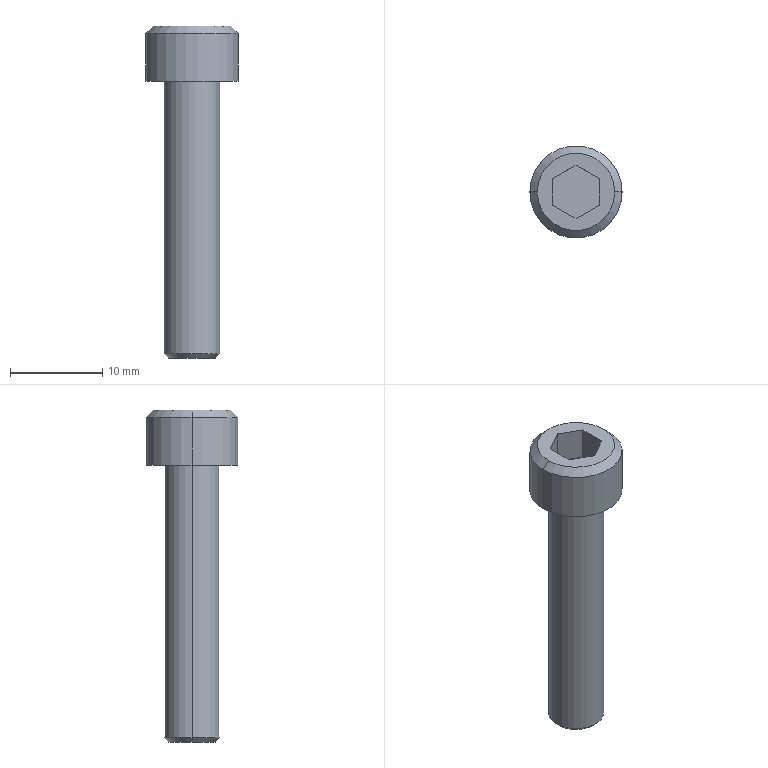Part | Creo | 1 solid | 18 faces | box 10 x 10 x 36 mm | volume 1230 mm3 | plane 10 | cylinder 4 | cone 4 | commonest cylinder face diameters 6 x2 10 x2
STEP:
#1=CARTESIAN_POINT('',(116.735,-194.,47.5));
#2=VERTEX_POINT('',#1);
#3=CARTESIAN_POINT('',(106.735,-194.,47.5));
#4=VERTEX_POINT('',#3);
#5=CARTESIAN_POINT('',(111.735,-194.,47.5));
#6=DIRECTION('',(0.,0.,-1.));
#7=DIRECTION('',(1.,0.,0.));
#8=AXIS2_PLACEMENT_3D('',#5,#6,#7);
#9=CIRCLE('',#8,5.);
#10=EDGE_CURVE('',#2,#4,#9,.T.);
#11=ORIENTED_EDGE('',*,*,#10,.F.);
#12=CARTESIAN_POINT('',(111.735,-194.,47.5));
#13=DIRECTION('',(0.,0.,-1.));
#14=DIRECTION('',(-1.,0.,0.));
#15=AXIS2_PLACEMENT_3D('',#12,#13,#14);
#16=CIRCLE('',#15,5.);
#17=EDGE_CURVE('',#4,#2,#16,.T.);
#18=ORIENTED_EDGE('',*,*,#17,.F.);
#19=EDGE_LOOP('',(#11,#18));
#20=FACE_OUTER_BOUND('',#19,.F.);
#21=CARTESIAN_POINT('',(108.735,-194.,47.5));
#22=VERTEX_POINT('',#21);
#23=CARTESIAN_POINT('',(114.735,-194.,47.5));
#24=VERTEX_POINT('',#23);
#25=CARTESIAN_POINT('',(111.735,-194.,47.5));
#26=DIRECTION('',(0.,0.,1.));
#27=DIRECTION('',(-1.,0.,0.));
#28=AXIS2_PLACEMENT_3D('',#25,#26,#27);
#29=CIRCLE('',#28,3.);
#30=EDGE_CURVE('',#22,#24,#29,.T.);
#31=ORIENTED_EDGE('',*,*,#30,.F.);
#32=CARTESIAN_POINT('',(111.735,-194.,47.5));
#33=DIRECTION('',(0.,0.,1.));
#34=DIRECTION('',(1.,0.,0.));
#35=AXIS2_PLACEMENT_3D('',#32,#33,#34);
#36=CIRCLE('',#35,3.);
#37=EDGE_CURVE('',#24,#22,#36,.T.);
#38=ORIENTED_EDGE('',*,*,#37,.F.);
#39=EDGE_LOOP('',(#31,#38));
#40=FACE_BOUND('',#39,.F.);
#41=CARTESIAN_POINT('',(111.735,-194.,47.5));
#42=DIRECTION('',(0.,0.,-1.));
#43=DIRECTION('',(-1.,0.,0.));
#44=AXIS2_PLACEMENT_3D('',#41,#42,#43);
#45=PLANE('',#44);
#46=ADVANCED_FACE('',(#20,#40),#45,.T.);
#47=CARTESIAN_POINT('',(114.735,-194.,17.95));
#48=VERTEX_POINT('',#47);
#49=CARTESIAN_POINT('',(108.735,-194.,17.95));
#50=VERTEX_POINT('',#49);
#51=CARTESIAN_POINT('',(111.735,-194.,17.95));
#52=DIRECTION('',(0.,0.,-1.));
#53=DIRECTION('',(1.,0.,0.));
#54=AXIS2_PLACEMENT_3D('',#51,#52,#53);
#55=CIRCLE('',#54,3.);
#56=EDGE_CURVE('',#48,#50,#55,.T.);
#57=ORIENTED_EDGE('',*,*,#56,.T.);
#58=CARTESIAN_POINT('',(108.735,-194.,47.5));
#59=DIRECTION('',(0.,0.,-1.));
#60=VECTOR('',#59,29.55);
#61=LINE('',#58,#60);
#62=EDGE_CURVE('',#22,#50,#61,.T.);
#63=ORIENTED_EDGE('',*,*,#62,.F.);
#64=ORIENTED_EDGE('',*,*,#30,.T.);
#65=CARTESIAN_POINT('',(114.735,-194.,47.5));
#66=DIRECTION('',(0.,0.,-1.));
#67=VECTOR('',#66,29.55);
#68=LINE('',#65,#67);
#69=EDGE_CURVE('',#24,#48,#68,.T.);
#70=ORIENTED_EDGE('',*,*,#69,.T.);
#71=EDGE_LOOP('',(#57,#63,#64,#70));
#72=FACE_OUTER_BOUND('',#71,.F.);
#73=CARTESIAN_POINT('',(111.735,-194.,54.5));
#74=DIRECTION('',(0.,0.,-1.));
#75=DIRECTION('',(-1.,0.,0.));
#76=AXIS2_PLACEMENT_3D('',#73,#74,#75);
#77=CYLINDRICAL_SURFACE('',#76,3.);
#78=ADVANCED_FACE('',(#72),#77,.T.);
#79=CARTESIAN_POINT('',(114.285,-194.,17.5));
#80=VERTEX_POINT('',#79);
#81=CARTESIAN_POINT('',(109.185,-194.,17.5));
#82=VERTEX_POINT('',#81);
#83=CARTESIAN_POINT('',(111.735,-194.,17.5));
#84=DIRECTION('',(0.,0.,-1.));
#85=DIRECTION('',(1.,0.,0.));
#86=AXIS2_PLACEMENT_3D('',#83,#84,#85);
#87=CIRCLE('',#86,2.55);
#88=EDGE_CURVE('',#80,#82,#87,.T.);
#89=ORIENTED_EDGE('',*,*,#88,.T.);
#90=CARTESIAN_POINT('',(109.185,-194.,17.5));
#91=DIRECTION('',(-0.7071,0.,0.7071));
#92=VECTOR('',#91,0.6364);
#93=LINE('',#90,#92);
#94=EDGE_CURVE('',#82,#50,#93,.T.);
#95=ORIENTED_EDGE('',*,*,#94,.T.);
#96=ORIENTED_EDGE('',*,*,#56,.F.);
#97=CARTESIAN_POINT('',(114.285,-194.,17.5));
#98=DIRECTION('',(0.7071,0.,0.7071));
#99=VECTOR('',#98,0.6364);
#100=LINE('',#97,#99);
#101=EDGE_CURVE('',#80,#48,#100,.T.);
#102=ORIENTED_EDGE('',*,*,#101,.F.);
#103=EDGE_LOOP('',(#89,#95,#96,#102));
#104=FACE_OUTER_BOUND('',#103,.F.);
#105=CARTESIAN_POINT('',(111.735,-194.,17.725));
#106=DIRECTION('',(0.,0.,1.));
#107=DIRECTION('',(1.,0.,0.));
#108=AXIS2_PLACEMENT_3D('',#105,#106,#107);
#109=CONICAL_SURFACE('',#108,2.775,45.);
#110=ADVANCED_FACE('',(#104),#109,.T.);
#111=CARTESIAN_POINT('',(111.735,-194.,17.5));
#112=DIRECTION('',(0.,0.,-1.));
#113=DIRECTION('',(-1.,0.,0.));
#114=AXIS2_PLACEMENT_3D('',#111,#112,#113);
#115=CIRCLE('',#114,2.55);
#116=EDGE_CURVE('',#82,#80,#115,.T.);
#117=ORIENTED_EDGE('',*,*,#116,.F.);
#118=ORIENTED_EDGE('',*,*,#88,.F.);
#119=EDGE_LOOP('',(#117,#118));
#120=FACE_OUTER_BOUND('',#119,.F.);
#121=CARTESIAN_POINT('',(111.735,-194.,17.5));
#122=DIRECTION('',(0.,0.,-1.));
#123=DIRECTION('',(-1.,0.,0.));
#124=AXIS2_PLACEMENT_3D('',#121,#122,#123);
#125=PLANE('',#124);
#126=ADVANCED_FACE('',(#120),#125,.T.);
#127=ORIENTED_EDGE('',*,*,#116,.T.);
#128=ORIENTED_EDGE('',*,*,#101,.T.);
#129=CARTESIAN_POINT('',(111.735,-194.,17.95));
#130=DIRECTION('',(0.,0.,-1.));
#131=DIRECTION('',(-1.,0.,0.));
#132=AXIS2_PLACEMENT_3D('',#129,#130,#131);
#133=CIRCLE('',#132,3.);
#134=EDGE_CURVE('',#50,#48,#133,.T.);
#135=ORIENTED_EDGE('',*,*,#134,.F.);
#136=ORIENTED_EDGE('',*,*,#94,.F.);
#137=EDGE_LOOP('',(#127,#128,#135,#136));
#138=FACE_OUTER_BOUND('',#137,.F.);
#139=CARTESIAN_POINT('',(111.735,-194.,17.725));
#140=DIRECTION('',(0.,0.,1.));
#141=DIRECTION('',(1.,0.,0.));
#142=AXIS2_PLACEMENT_3D('',#139,#140,#141);
#143=CONICAL_SURFACE('',#142,2.775,45.);
#144=ADVANCED_FACE('',(#138),#143,.T.);
#145=ORIENTED_EDGE('',*,*,#134,.T.);
#146=ORIENTED_EDGE('',*,*,#69,.F.);
#147=ORIENTED_EDGE('',*,*,#37,.T.);
#148=ORIENTED_EDGE('',*,*,#62,.T.);
#149=EDGE_LOOP('',(#145,#146,#147,#148));
#150=FACE_OUTER_BOUND('',#149,.F.);
#151=CARTESIAN_POINT('',(111.735,-194.,54.5));
#152=DIRECTION('',(0.,0.,-1.));
#153=DIRECTION('',(-1.,0.,0.));
#154=AXIS2_PLACEMENT_3D('',#151,#152,#153);
#155=CYLINDRICAL_SURFACE('',#154,3.);
#156=ADVANCED_FACE('',(#150),#155,.T.);
#157=CARTESIAN_POINT('',(106.735,-194.,52.7));
#158=VERTEX_POINT('',#157);
#159=CARTESIAN_POINT('',(116.735,-194.,52.7));
#160=VERTEX_POINT('',#159);
#161=CARTESIAN_POINT('',(111.735,-194.,52.7));
#162=DIRECTION('',(0.,0.,1.));
#163=DIRECTION('',(-1.,0.,0.));
#164=AXIS2_PLACEMENT_3D('',#161,#162,#163);
#165=CIRCLE('',#164,5.);
#166=EDGE_CURVE('',#158,#160,#165,.T.);
#167=ORIENTED_EDGE('',*,*,#166,.T.);
#168=CARTESIAN_POINT('',(116.735,-194.,52.7));
#169=DIRECTION('',(0.,0.,-1.));
#170=VECTOR('',#169,5.2);
#171=LINE('',#168,#170);
#172=EDGE_CURVE('',#160,#2,#171,.T.);
#173=ORIENTED_EDGE('',*,*,#172,.T.);
#174=ORIENTED_EDGE('',*,*,#10,.T.);
#175=CARTESIAN_POINT('',(106.735,-194.,52.7));
#176=DIRECTION('',(0.,0.,-1.));
#177=VECTOR('',#176,5.2);
#178=LINE('',#175,#177);
#179=EDGE_CURVE('',#158,#4,#178,.T.);
#180=ORIENTED_EDGE('',*,*,#179,.F.);
#181=EDGE_LOOP('',(#167,#173,#174,#180));
#182=FACE_OUTER_BOUND('',#181,.F.);
#183=CARTESIAN_POINT('',(111.735,-194.,54.5));
#184=DIRECTION('',(0.,0.,-1.));
#185=DIRECTION('',(-1.,0.,0.));
#186=AXIS2_PLACEMENT_3D('',#183,#184,#185);
#187=CYLINDRICAL_SURFACE('',#186,5.);
#188=ADVANCED_FACE('',(#182),#187,.T.);
#189=CARTESIAN_POINT('',(107.535,-194.,53.5));
#190=VERTEX_POINT('',#189);
#191=CARTESIAN_POINT('',(115.935,-194.,53.5));
#192=VERTEX_POINT('',#191);
#193=CARTESIAN_POINT('',(111.735,-194.,53.5));
#194=DIRECTION('',(0.,0.,1.));
#195=DIRECTION('',(-1.,0.,0.));
#196=AXIS2_PLACEMENT_3D('',#193,#194,#195);
#197=CIRCLE('',#196,4.2);
#198=EDGE_CURVE('',#190,#192,#197,.T.);
#199=ORIENTED_EDGE('',*,*,#198,.T.);
#200=CARTESIAN_POINT('',(115.935,-194.,53.5));
#201=DIRECTION('',(0.7071,0.,-0.7071));
#202=VECTOR('',#201,1.131);
#203=LINE('',#200,#202);
#204=EDGE_CURVE('',#192,#160,#203,.T.);
#205=ORIENTED_EDGE('',*,*,#204,.T.);
#206=ORIENTED_EDGE('',*,*,#166,.F.);
#207=CARTESIAN_POINT('',(107.535,-194.,53.5));
#208=DIRECTION('',(-0.7071,0.,-0.7071));
#209=VECTOR('',#208,1.131);
#210=LINE('',#207,#209);
#211=EDGE_CURVE('',#190,#158,#210,.T.);
#212=ORIENTED_EDGE('',*,*,#211,.F.);
#213=EDGE_LOOP('',(#199,#205,#206,#212));
#214=FACE_OUTER_BOUND('',#213,.F.);
#215=CARTESIAN_POINT('',(111.735,-194.,53.1));
#216=DIRECTION('',(0.,0.,-1.));
#217=DIRECTION('',(-1.,0.,0.));
#218=AXIS2_PLACEMENT_3D('',#215,#216,#217);
#219=CONICAL_SURFACE('',#218,4.6,45.);
#220=ADVANCED_FACE('',(#214),#219,.T.);
#221=ORIENTED_EDGE('',*,*,#198,.F.);
#222=CARTESIAN_POINT('',(111.735,-194.,53.5));
#223=DIRECTION('',(0.,0.,1.));
#224=DIRECTION('',(1.,0.,0.));
#225=AXIS2_PLACEMENT_3D('',#222,#223,#224);
#226=CIRCLE('',#225,4.2);
#227=EDGE_CURVE('',#192,#190,#226,.T.);
#228=ORIENTED_EDGE('',*,*,#227,.F.);
#229=EDGE_LOOP('',(#221,#228));
#230=FACE_OUTER_BOUND('',#229,.F.);
#231=CARTESIAN_POINT('',(114.235,-195.443,53.5));
#232=VERTEX_POINT('',#231);
#233=CARTESIAN_POINT('',(111.735,-196.887,53.5));
#234=VERTEX_POINT('',#233);
#235=CARTESIAN_POINT('',(114.235,-195.443,53.5));
#236=DIRECTION('',(-0.866,-0.5,0.));
#237=VECTOR('',#236,2.887);
#238=LINE('',#235,#237);
#239=EDGE_CURVE('',#232,#234,#238,.T.);
#240=ORIENTED_EDGE('',*,*,#239,.F.);
#241=CARTESIAN_POINT('',(114.235,-192.557,53.5));
#242=VERTEX_POINT('',#241);
#243=CARTESIAN_POINT('',(114.235,-192.557,53.5));
#244=DIRECTION('',(0.,-1.,0.));
#245=VECTOR('',#244,2.887);
#246=LINE('',#243,#245);
#247=EDGE_CURVE('',#242,#232,#246,.T.);
#248=ORIENTED_EDGE('',*,*,#247,.F.);
#249=CARTESIAN_POINT('',(111.735,-191.113,53.5));
#250=VERTEX_POINT('',#249);
#251=CARTESIAN_POINT('',(111.735,-191.113,53.5));
#252=DIRECTION('',(0.866,-0.5,0.));
#253=VECTOR('',#252,2.887);
#254=LINE('',#251,#253);
#255=EDGE_CURVE('',#250,#242,#254,.T.);
#256=ORIENTED_EDGE('',*,*,#255,.F.);
#257=CARTESIAN_POINT('',(109.235,-192.557,53.5));
#258=VERTEX_POINT('',#257);
#259=CARTESIAN_POINT('',(109.235,-192.557,53.5));
#260=DIRECTION('',(0.866,0.5,0.));
#261=VECTOR('',#260,2.887);
#262=LINE('',#259,#261);
#263=EDGE_CURVE('',#258,#250,#262,.T.);
#264=ORIENTED_EDGE('',*,*,#263,.F.);
#265=CARTESIAN_POINT('',(109.235,-195.443,53.5));
#266=VERTEX_POINT('',#265);
#267=CARTESIAN_POINT('',(109.235,-195.443,53.5));
#268=DIRECTION('',(0.,1.,0.));
#269=VECTOR('',#268,2.887);
#270=LINE('',#267,#269);
#271=EDGE_CURVE('',#266,#258,#270,.T.);
#272=ORIENTED_EDGE('',*,*,#271,.F.);
#273=CARTESIAN_POINT('',(111.735,-196.887,53.5));
#274=DIRECTION('',(-0.866,0.5,0.));
#275=VECTOR('',#274,2.887);
#276=LINE('',#273,#275);
#277=EDGE_CURVE('',#234,#266,#276,.T.);
#278=ORIENTED_EDGE('',*,*,#277,.F.);
#279=EDGE_LOOP('',(#240,#248,#256,#264,#272,#278));
#280=FACE_BOUND('',#279,.F.);
#281=CARTESIAN_POINT('',(111.735,-194.,53.5));
#282=DIRECTION('',(0.,0.,-1.));
#283=DIRECTION('',(-1.,0.,0.));
#284=AXIS2_PLACEMENT_3D('',#281,#282,#283);
#285=PLANE('',#284);
#286=ADVANCED_FACE('',(#230,#280),#285,.F.);
#287=ORIENTED_EDGE('',*,*,#227,.T.);
#288=ORIENTED_EDGE('',*,*,#211,.T.);
#289=CARTESIAN_POINT('',(111.735,-194.,52.7));
#290=DIRECTION('',(0.,0.,1.));
#291=DIRECTION('',(1.,0.,0.));
#292=AXIS2_PLACEMENT_3D('',#289,#290,#291);
#293=CIRCLE('',#292,5.);
#294=EDGE_CURVE('',#160,#158,#293,.T.);
#295=ORIENTED_EDGE('',*,*,#294,.F.);
#296=ORIENTED_EDGE('',*,*,#204,.F.);
#297=EDGE_LOOP('',(#287,#288,#295,#296));
#298=FACE_OUTER_BOUND('',#297,.F.);
#299=CARTESIAN_POINT('',(111.735,-194.,53.1));
#300=DIRECTION('',(0.,0.,-1.));
#301=DIRECTION('',(-1.,0.,0.));
#302=AXIS2_PLACEMENT_3D('',#299,#300,#301);
#303=CONICAL_SURFACE('',#302,4.6,45.);
#304=ADVANCED_FACE('',(#298),#303,.T.);
#305=ORIENTED_EDGE('',*,*,#294,.T.);
#306=ORIENTED_EDGE('',*,*,#179,.T.);
#307=ORIENTED_EDGE('',*,*,#17,.T.);
#308=ORIENTED_EDGE('',*,*,#172,.F.);
#309=EDGE_LOOP('',(#305,#306,#307,#308));
#310=FACE_OUTER_BOUND('',#309,.F.);
#311=CARTESIAN_POINT('',(111.735,-194.,54.5));
#312=DIRECTION('',(0.,0.,-1.));
#313=DIRECTION('',(-1.,0.,0.));
#314=AXIS2_PLACEMENT_3D('',#311,#312,#313);
#315=CYLINDRICAL_SURFACE('',#314,5.);
#316=ADVANCED_FACE('',(#310),#315,.T.);
#317=ORIENTED_EDGE('',*,*,#239,.T.);
#318=CARTESIAN_POINT('',(111.735,-196.887,49.9));
#319=VERTEX_POINT('',#318);
#320=CARTESIAN_POINT('',(111.735,-196.887,53.5));
#321=DIRECTION('',(0.,0.,-1.));
#322=VECTOR('',#321,3.6);
#323=LINE('',#320,#322);
#324=EDGE_CURVE('',#234,#319,#323,.T.);
#325=ORIENTED_EDGE('',*,*,#324,.T.);
#326=CARTESIAN_POINT('',(114.235,-195.443,49.9));
#327=VERTEX_POINT('',#326);
#328=CARTESIAN_POINT('',(111.735,-196.887,49.9));
#329=DIRECTION('',(0.866,0.5,0.));
#330=VECTOR('',#329,2.887);
#331=LINE('',#328,#330);
#332=EDGE_CURVE('',#319,#327,#331,.T.);
#333=ORIENTED_EDGE('',*,*,#332,.T.);
#334=CARTESIAN_POINT('',(114.235,-195.443,53.5));
#335=DIRECTION('',(0.,0.,-1.));
#336=VECTOR('',#335,3.6);
#337=LINE('',#334,#336);
#338=EDGE_CURVE('',#232,#327,#337,.T.);
#339=ORIENTED_EDGE('',*,*,#338,.F.);
#340=EDGE_LOOP('',(#317,#325,#333,#339));
#341=FACE_OUTER_BOUND('',#340,.F.);
#342=CARTESIAN_POINT('',(111.735,-196.887,49.9));
#343=DIRECTION('',(0.5,-0.866,0.));
#344=DIRECTION('',(0.866,0.5,0.));
#345=AXIS2_PLACEMENT_3D('',#342,#343,#344);
#346=PLANE('',#345);
#347=ADVANCED_FACE('',(#341),#346,.F.);
#348=ORIENTED_EDGE('',*,*,#277,.T.);
#349=CARTESIAN_POINT('',(109.235,-195.443,49.9));
#350=VERTEX_POINT('',#349);
#351=CARTESIAN_POINT('',(109.235,-195.443,53.5));
#352=DIRECTION('',(0.,0.,-1.));
#353=VECTOR('',#352,3.6);
#354=LINE('',#351,#353);
#355=EDGE_CURVE('',#266,#350,#354,.T.);
#356=ORIENTED_EDGE('',*,*,#355,.T.);
#357=CARTESIAN_POINT('',(109.235,-195.443,49.9));
#358=DIRECTION('',(0.866,-0.5,0.));
#359=VECTOR('',#358,2.887);
#360=LINE('',#357,#359);
#361=EDGE_CURVE('',#350,#319,#360,.T.);
#362=ORIENTED_EDGE('',*,*,#361,.T.);
#363=ORIENTED_EDGE('',*,*,#324,.F.);
#364=EDGE_LOOP('',(#348,#356,#362,#363));
#365=FACE_OUTER_BOUND('',#364,.F.);
#366=CARTESIAN_POINT('',(109.235,-195.443,49.9));
#367=DIRECTION('',(-0.5,-0.866,0.));
#368=DIRECTION('',(0.866,-0.5,0.));
#369=AXIS2_PLACEMENT_3D('',#366,#367,#368);
#370=PLANE('',#369);
#371=ADVANCED_FACE('',(#365),#370,.F.);
#372=ORIENTED_EDGE('',*,*,#271,.T.);
#373=CARTESIAN_POINT('',(109.235,-192.557,49.9));
#374=VERTEX_POINT('',#373);
#375=CARTESIAN_POINT('',(109.235,-192.557,53.5));
#376=DIRECTION('',(0.,0.,-1.));
#377=VECTOR('',#376,3.6);
#378=LINE('',#375,#377);
#379=EDGE_CURVE('',#258,#374,#378,.T.);
#380=ORIENTED_EDGE('',*,*,#379,.T.);
#381=CARTESIAN_POINT('',(109.235,-195.443,49.9));
#382=DIRECTION('',(0.,1.,0.));
#383=VECTOR('',#382,2.887);
#384=LINE('',#381,#383);
#385=EDGE_CURVE('',#350,#374,#384,.T.);
#386=ORIENTED_EDGE('',*,*,#385,.F.);
#387=ORIENTED_EDGE('',*,*,#355,.F.);
#388=EDGE_LOOP('',(#372,#380,#386,#387));
#389=FACE_OUTER_BOUND('',#388,.F.);
#390=CARTESIAN_POINT('',(109.235,-192.557,49.9));
#391=DIRECTION('',(-1.,0.,0.));
#392=DIRECTION('',(0.,0.,1.));
#393=AXIS2_PLACEMENT_3D('',#390,#391,#392);
#394=PLANE('',#393);
#395=ADVANCED_FACE('',(#389),#394,.F.);
#396=ORIENTED_EDGE('',*,*,#263,.T.);
#397=CARTESIAN_POINT('',(111.735,-191.113,49.9));
#398=VERTEX_POINT('',#397);
#399=CARTESIAN_POINT('',(111.735,-191.113,53.5));
#400=DIRECTION('',(0.,0.,-1.));
#401=VECTOR('',#400,3.6);
#402=LINE('',#399,#401);
#403=EDGE_CURVE('',#250,#398,#402,.T.);
#404=ORIENTED_EDGE('',*,*,#403,.T.);
#405=CARTESIAN_POINT('',(111.735,-191.113,49.9));
#406=DIRECTION('',(-0.866,-0.5,0.));
#407=VECTOR('',#406,2.887);
#408=LINE('',#405,#407);
#409=EDGE_CURVE('',#398,#374,#408,.T.);
#410=ORIENTED_EDGE('',*,*,#409,.T.);
#411=ORIENTED_EDGE('',*,*,#379,.F.);
#412=EDGE_LOOP('',(#396,#404,#410,#411));
#413=FACE_OUTER_BOUND('',#412,.F.);
#414=CARTESIAN_POINT('',(111.735,-191.113,49.9));
#415=DIRECTION('',(-0.5,0.866,0.));
#416=DIRECTION('',(-0.866,-0.5,0.));
#417=AXIS2_PLACEMENT_3D('',#414,#415,#416);
#418=PLANE('',#417);
#419=ADVANCED_FACE('',(#413),#418,.F.);
#420=ORIENTED_EDGE('',*,*,#255,.T.);
#421=CARTESIAN_POINT('',(114.235,-192.557,49.9));
#422=VERTEX_POINT('',#421);
#423=CARTESIAN_POINT('',(114.235,-192.557,53.5));
#424=DIRECTION('',(0.,0.,-1.));
#425=VECTOR('',#424,3.6);
#426=LINE('',#423,#425);
#427=EDGE_CURVE('',#242,#422,#426,.T.);
#428=ORIENTED_EDGE('',*,*,#427,.T.);
#429=CARTESIAN_POINT('',(114.235,-192.557,49.9));
#430=DIRECTION('',(-0.866,0.5,0.));
#431=VECTOR('',#430,2.887);
#432=LINE('',#429,#431);
#433=EDGE_CURVE('',#422,#398,#432,.T.);
#434=ORIENTED_EDGE('',*,*,#433,.T.);
#435=ORIENTED_EDGE('',*,*,#403,.F.);
#436=EDGE_LOOP('',(#420,#428,#434,#435));
#437=FACE_OUTER_BOUND('',#436,.F.);
#438=CARTESIAN_POINT('',(114.235,-192.557,49.9));
#439=DIRECTION('',(0.5,0.866,0.));
#440=DIRECTION('',(-0.866,0.5,0.));
#441=AXIS2_PLACEMENT_3D('',#438,#439,#440);
#442=PLANE('',#441);
#443=ADVANCED_FACE('',(#437),#442,.F.);
#444=ORIENTED_EDGE('',*,*,#247,.T.);
#445=ORIENTED_EDGE('',*,*,#338,.T.);
#446=CARTESIAN_POINT('',(114.235,-192.557,49.9));
#447=DIRECTION('',(0.,-1.,0.));
#448=VECTOR('',#447,2.887);
#449=LINE('',#446,#448);
#450=EDGE_CURVE('',#422,#327,#449,.T.);
#451=ORIENTED_EDGE('',*,*,#450,.F.);
#452=ORIENTED_EDGE('',*,*,#427,.F.);
#453=EDGE_LOOP('',(#444,#445,#451,#452));
#454=FACE_OUTER_BOUND('',#453,.F.);
#455=CARTESIAN_POINT('',(114.235,-195.443,49.9));
#456=DIRECTION('',(1.,0.,0.));
#457=DIRECTION('',(0.,0.,-1.));
#458=AXIS2_PLACEMENT_3D('',#455,#456,#457);
#459=PLANE('',#458);
#460=ADVANCED_FACE('',(#454),#459,.F.);
#461=ORIENTED_EDGE('',*,*,#361,.F.);
#462=ORIENTED_EDGE('',*,*,#385,.T.);
#463=ORIENTED_EDGE('',*,*,#409,.F.);
#464=ORIENTED_EDGE('',*,*,#433,.F.);
#465=ORIENTED_EDGE('',*,*,#450,.T.);
#466=ORIENTED_EDGE('',*,*,#332,.F.);
#467=EDGE_LOOP('',(#461,#462,#463,#464,#465,#466));
#468=FACE_OUTER_BOUND('',#467,.F.);
#469=CARTESIAN_POINT('',(114.235,-198.33,49.9));
#470=DIRECTION('',(0.,0.,1.));
#471=DIRECTION('',(0.,-1.,0.));
#472=AXIS2_PLACEMENT_3D('',#469,#470,#471);
#473=PLANE('',#472);
#474=ADVANCED_FACE('',(#468),#473,.T.);
#475=CLOSED_SHELL('',(#46,#78,#110,#126,#144,#156,#188,#220,#286,#304,#316,#347,#371,#395,#419,#443,#460,#474));
#476=MANIFOLD_SOLID_BREP('',#475);
#477=(LENGTH_UNIT()NAMED_UNIT(*)SI_UNIT(.MILLI.,.METRE.));
#478=UNCERTAINTY_MEASURE_WITH_UNIT(LENGTH_MEASURE(0.003868),#477,'','');
#479=(NAMED_UNIT(*)PLANE_ANGLE_UNIT()SI_UNIT($,.RADIAN.));
#480=PLANE_ANGLE_MEASURE_WITH_UNIT(PLANE_ANGLE_MEASURE(0.01745),#479);
#481=(CONVERSION_BASED_UNIT('DEGREE',#480)NAMED_UNIT(*)PLANE_ANGLE_UNIT());
#482=(NAMED_UNIT(*)SI_UNIT($,.STERADIAN.)SOLID_ANGLE_UNIT());
#483=(GEOMETRIC_REPRESENTATION_CONTEXT(3)GLOBAL_UNCERTAINTY_ASSIGNED_CONTEXT((#478))GLOBAL_UNIT_ASSIGNED_CONTEXT((#477,#481,#482))REPRESENTATION_CONTEXT('',''));
#484=ADVANCED_BREP_SHAPE_REPRESENTATION('',(#476),#483);